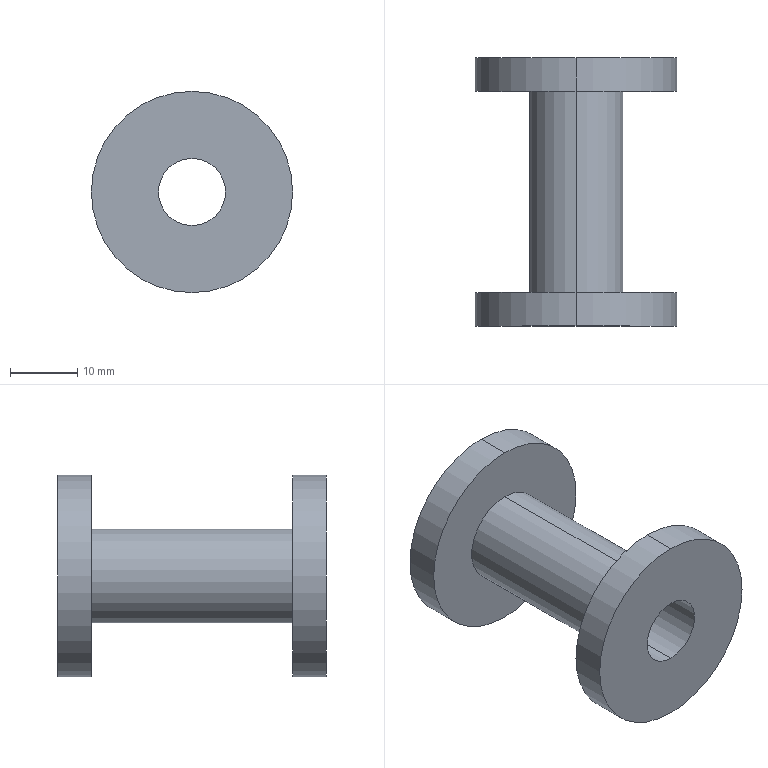Part | STEP file | inner coil1 | 1 solid | 12 faces | box 30 x 40 x 30 mm | volume 8545 mm3 | cylinder 8 | plane 4 | commonest cylinder face diameters 30 x4 10 x2 14 x2
STEP:
#1=CARTESIAN_POINT('',(0.,-15.,7.));
#2=VERTEX_POINT('',#1);
#3=CARTESIAN_POINT('',(0.,-15.,-7.));
#4=VERTEX_POINT('',#3);
#5=CARTESIAN_POINT('',(0.,-15.,0.));
#6=DIRECTION('',(0.,1.,0.));
#7=DIRECTION('',(0.,0.,1.));
#8=AXIS2_PLACEMENT_3D('',#5,#6,#7);
#9=CIRCLE('',#8,7.);
#10=EDGE_CURVE('',#2,#4,#9,.T.);
#11=ORIENTED_EDGE('',*,*,#10,.T.);
#12=CARTESIAN_POINT('',(0.,15.,-7.));
#13=VERTEX_POINT('',#12);
#14=CARTESIAN_POINT('',(0.,13.555,-7.));
#15=DIRECTION('',(0.,1.,0.));
#16=VECTOR('',#15,1000.);
#17=LINE('',#14,#16);
#18=EDGE_CURVE('',#4,#13,#17,.T.);
#19=ORIENTED_EDGE('',*,*,#18,.T.);
#20=CARTESIAN_POINT('',(0.,15.,7.));
#21=VERTEX_POINT('',#20);
#22=CARTESIAN_POINT('',(0.,15.,0.));
#23=DIRECTION('',(0.,1.,0.));
#24=DIRECTION('',(0.,0.,1.));
#25=AXIS2_PLACEMENT_3D('',#22,#23,#24);
#26=CIRCLE('',#25,7.);
#27=EDGE_CURVE('',#21,#13,#26,.T.);
#28=ORIENTED_EDGE('',*,*,#27,.F.);
#29=CARTESIAN_POINT('',(0.,13.555,7.));
#30=DIRECTION('',(0.,1.,0.));
#31=VECTOR('',#30,1000.);
#32=LINE('',#29,#31);
#33=EDGE_CURVE('',#2,#21,#32,.T.);
#34=ORIENTED_EDGE('',*,*,#33,.F.);
#35=EDGE_LOOP('',(#11,#19,#28,#34));
#36=FACE_OUTER_BOUND('',#35,.T.);
#37=CARTESIAN_POINT('',(0.,13.555,0.));
#38=DIRECTION('',(0.,1.,0.));
#39=DIRECTION('',(0.,0.,1.));
#40=AXIS2_PLACEMENT_3D('',#37,#38,#39);
#41=CYLINDRICAL_SURFACE('',#40,7.);
#42=ADVANCED_FACE('',(#36),#41,.T.);
#43=CARTESIAN_POINT('',(0.,-20.,-5.));
#44=VERTEX_POINT('',#43);
#45=CARTESIAN_POINT('',(0.,-20.,5.));
#46=VERTEX_POINT('',#45);
#47=CARTESIAN_POINT('',(0.,-20.,0.));
#48=DIRECTION('',(0.,1.,0.));
#49=DIRECTION('',(0.,0.,1.));
#50=AXIS2_PLACEMENT_3D('',#47,#48,#49);
#51=CIRCLE('',#50,5.);
#52=EDGE_CURVE('',#44,#46,#51,.T.);
#53=ORIENTED_EDGE('',*,*,#52,.F.);
#54=CARTESIAN_POINT('',(0.,20.,-5.));
#55=VERTEX_POINT('',#54);
#56=CARTESIAN_POINT('',(0.,65.771,-5.));
#57=DIRECTION('',(0.,1.,0.));
#58=VECTOR('',#57,1000.);
#59=LINE('',#56,#58);
#60=EDGE_CURVE('',#44,#55,#59,.T.);
#61=ORIENTED_EDGE('',*,*,#60,.T.);
#62=CARTESIAN_POINT('',(0.,20.,5.));
#63=VERTEX_POINT('',#62);
#64=CARTESIAN_POINT('',(0.,20.,0.));
#65=DIRECTION('',(0.,1.,0.));
#66=DIRECTION('',(0.,0.,1.));
#67=AXIS2_PLACEMENT_3D('',#64,#65,#66);
#68=CIRCLE('',#67,5.);
#69=EDGE_CURVE('',#55,#63,#68,.T.);
#70=ORIENTED_EDGE('',*,*,#69,.T.);
#71=CARTESIAN_POINT('',(0.,65.771,5.));
#72=DIRECTION('',(0.,1.,0.));
#73=VECTOR('',#72,1000.);
#74=LINE('',#71,#73);
#75=EDGE_CURVE('',#46,#63,#74,.T.);
#76=ORIENTED_EDGE('',*,*,#75,.F.);
#77=EDGE_LOOP('',(#53,#61,#70,#76));
#78=FACE_OUTER_BOUND('',#77,.T.);
#79=CARTESIAN_POINT('',(0.,65.771,0.));
#80=DIRECTION('',(0.,1.,0.));
#81=DIRECTION('',(0.,0.,1.));
#82=AXIS2_PLACEMENT_3D('',#79,#80,#81);
#83=CYLINDRICAL_SURFACE('',#82,5.);
#84=ADVANCED_FACE('',(#78),#83,.F.);
#85=CARTESIAN_POINT('',(0.,15.,15.));
#86=VERTEX_POINT('',#85);
#87=CARTESIAN_POINT('',(0.,15.,-15.));
#88=VERTEX_POINT('',#87);
#89=CARTESIAN_POINT('',(0.,15.,0.));
#90=DIRECTION('',(0.,1.,0.));
#91=DIRECTION('',(0.,0.,1.));
#92=AXIS2_PLACEMENT_3D('',#89,#90,#91);
#93=CIRCLE('',#92,15.);
#94=EDGE_CURVE('',#86,#88,#93,.T.);
#95=ORIENTED_EDGE('',*,*,#94,.T.);
#96=CARTESIAN_POINT('',(0.,20.,-15.));
#97=VERTEX_POINT('',#96);
#98=CARTESIAN_POINT('',(0.,65.771,-15.));
#99=DIRECTION('',(0.,1.,0.));
#100=VECTOR('',#99,1000.);
#101=LINE('',#98,#100);
#102=EDGE_CURVE('',#88,#97,#101,.T.);
#103=ORIENTED_EDGE('',*,*,#102,.T.);
#104=CARTESIAN_POINT('',(0.,20.,15.));
#105=VERTEX_POINT('',#104);
#106=CARTESIAN_POINT('',(0.,20.,0.));
#107=DIRECTION('',(0.,1.,0.));
#108=DIRECTION('',(0.,0.,1.));
#109=AXIS2_PLACEMENT_3D('',#106,#107,#108);
#110=CIRCLE('',#109,15.);
#111=EDGE_CURVE('',#105,#97,#110,.T.);
#112=ORIENTED_EDGE('',*,*,#111,.F.);
#113=CARTESIAN_POINT('',(0.,65.771,15.));
#114=DIRECTION('',(0.,1.,0.));
#115=VECTOR('',#114,1000.);
#116=LINE('',#113,#115);
#117=EDGE_CURVE('',#86,#105,#116,.T.);
#118=ORIENTED_EDGE('',*,*,#117,.F.);
#119=EDGE_LOOP('',(#95,#103,#112,#118));
#120=FACE_OUTER_BOUND('',#119,.T.);
#121=CARTESIAN_POINT('',(0.,65.771,0.));
#122=DIRECTION('',(0.,1.,0.));
#123=DIRECTION('',(0.,0.,1.));
#124=AXIS2_PLACEMENT_3D('',#121,#122,#123);
#125=CYLINDRICAL_SURFACE('',#124,15.);
#126=ADVANCED_FACE('',(#120),#125,.T.);
#127=CARTESIAN_POINT('',(0.,-20.,15.));
#128=VERTEX_POINT('',#127);
#129=CARTESIAN_POINT('',(0.,-20.,-15.));
#130=VERTEX_POINT('',#129);
#131=CARTESIAN_POINT('',(0.,-20.,0.));
#132=DIRECTION('',(0.,1.,0.));
#133=DIRECTION('',(0.,0.,1.));
#134=AXIS2_PLACEMENT_3D('',#131,#132,#133);
#135=CIRCLE('',#134,15.);
#136=EDGE_CURVE('',#128,#130,#135,.T.);
#137=ORIENTED_EDGE('',*,*,#136,.T.);
#138=CARTESIAN_POINT('',(0.,-15.,-15.));
#139=VERTEX_POINT('',#138);
#140=CARTESIAN_POINT('',(0.,65.771,-15.));
#141=DIRECTION('',(0.,1.,0.));
#142=VECTOR('',#141,1000.);
#143=LINE('',#140,#142);
#144=EDGE_CURVE('',#130,#139,#143,.T.);
#145=ORIENTED_EDGE('',*,*,#144,.T.);
#146=CARTESIAN_POINT('',(0.,-15.,15.));
#147=VERTEX_POINT('',#146);
#148=CARTESIAN_POINT('',(0.,-15.,0.));
#149=DIRECTION('',(0.,1.,0.));
#150=DIRECTION('',(0.,0.,1.));
#151=AXIS2_PLACEMENT_3D('',#148,#149,#150);
#152=CIRCLE('',#151,15.);
#153=EDGE_CURVE('',#147,#139,#152,.T.);
#154=ORIENTED_EDGE('',*,*,#153,.F.);
#155=CARTESIAN_POINT('',(0.,65.771,15.));
#156=DIRECTION('',(0.,1.,0.));
#157=VECTOR('',#156,1000.);
#158=LINE('',#155,#157);
#159=EDGE_CURVE('',#128,#147,#158,.T.);
#160=ORIENTED_EDGE('',*,*,#159,.F.);
#161=EDGE_LOOP('',(#137,#145,#154,#160));
#162=FACE_OUTER_BOUND('',#161,.T.);
#163=CARTESIAN_POINT('',(0.,65.771,0.));
#164=DIRECTION('',(0.,1.,0.));
#165=DIRECTION('',(0.,0.,1.));
#166=AXIS2_PLACEMENT_3D('',#163,#164,#165);
#167=CYLINDRICAL_SURFACE('',#166,15.);
#168=ADVANCED_FACE('',(#162),#167,.T.);
#169=ORIENTED_EDGE('',*,*,#144,.F.);
#170=CARTESIAN_POINT('',(0.,-20.,0.));
#171=DIRECTION('',(0.,1.,0.));
#172=DIRECTION('',(0.,0.,1.));
#173=AXIS2_PLACEMENT_3D('',#170,#171,#172);
#174=CIRCLE('',#173,15.);
#175=EDGE_CURVE('',#130,#128,#174,.T.);
#176=ORIENTED_EDGE('',*,*,#175,.T.);
#177=ORIENTED_EDGE('',*,*,#159,.T.);
#178=CARTESIAN_POINT('',(0.,-15.,0.));
#179=DIRECTION('',(0.,1.,0.));
#180=DIRECTION('',(0.,0.,1.));
#181=AXIS2_PLACEMENT_3D('',#178,#179,#180);
#182=CIRCLE('',#181,15.);
#183=EDGE_CURVE('',#139,#147,#182,.T.);
#184=ORIENTED_EDGE('',*,*,#183,.F.);
#185=EDGE_LOOP('',(#169,#176,#177,#184));
#186=FACE_OUTER_BOUND('',#185,.T.);
#187=CARTESIAN_POINT('',(0.,65.771,0.));
#188=DIRECTION('',(0.,1.,0.));
#189=DIRECTION('',(0.,0.,1.));
#190=AXIS2_PLACEMENT_3D('',#187,#188,#189);
#191=CYLINDRICAL_SURFACE('',#190,15.);
#192=ADVANCED_FACE('',(#186),#191,.T.);
#193=ORIENTED_EDGE('',*,*,#102,.F.);
#194=CARTESIAN_POINT('',(0.,15.,0.));
#195=DIRECTION('',(0.,1.,0.));
#196=DIRECTION('',(0.,0.,1.));
#197=AXIS2_PLACEMENT_3D('',#194,#195,#196);
#198=CIRCLE('',#197,15.);
#199=EDGE_CURVE('',#88,#86,#198,.T.);
#200=ORIENTED_EDGE('',*,*,#199,.T.);
#201=ORIENTED_EDGE('',*,*,#117,.T.);
#202=CARTESIAN_POINT('',(0.,20.,0.));
#203=DIRECTION('',(0.,1.,0.));
#204=DIRECTION('',(0.,0.,1.));
#205=AXIS2_PLACEMENT_3D('',#202,#203,#204);
#206=CIRCLE('',#205,15.);
#207=EDGE_CURVE('',#97,#105,#206,.T.);
#208=ORIENTED_EDGE('',*,*,#207,.F.);
#209=EDGE_LOOP('',(#193,#200,#201,#208));
#210=FACE_OUTER_BOUND('',#209,.T.);
#211=CARTESIAN_POINT('',(0.,65.771,0.));
#212=DIRECTION('',(0.,1.,0.));
#213=DIRECTION('',(0.,0.,1.));
#214=AXIS2_PLACEMENT_3D('',#211,#212,#213);
#215=CYLINDRICAL_SURFACE('',#214,15.);
#216=ADVANCED_FACE('',(#210),#215,.T.);
#217=ORIENTED_EDGE('',*,*,#111,.T.);
#218=ORIENTED_EDGE('',*,*,#207,.T.);
#219=EDGE_LOOP('',(#217,#218));
#220=FACE_OUTER_BOUND('',#219,.T.);
#221=CARTESIAN_POINT('',(0.,20.,0.));
#222=DIRECTION('',(0.,1.,0.));
#223=DIRECTION('',(0.,0.,1.));
#224=AXIS2_PLACEMENT_3D('',#221,#222,#223);
#225=CIRCLE('',#224,5.);
#226=EDGE_CURVE('',#63,#55,#225,.T.);
#227=ORIENTED_EDGE('',*,*,#226,.F.);
#228=ORIENTED_EDGE('',*,*,#69,.F.);
#229=EDGE_LOOP('',(#227,#228));
#230=FACE_BOUND('',#229,.T.);
#231=CARTESIAN_POINT('',(-5.,20.,0.));
#232=DIRECTION('',(0.,1.,0.));
#233=DIRECTION('',(0.,0.,1.));
#234=AXIS2_PLACEMENT_3D('',#231,#232,#233);
#235=PLANE('',#234);
#236=ADVANCED_FACE('',(#220,#230),#235,.T.);
#237=ORIENTED_EDGE('',*,*,#60,.F.);
#238=CARTESIAN_POINT('',(0.,-20.,0.));
#239=DIRECTION('',(0.,1.,0.));
#240=DIRECTION('',(0.,0.,1.));
#241=AXIS2_PLACEMENT_3D('',#238,#239,#240);
#242=CIRCLE('',#241,5.);
#243=EDGE_CURVE('',#46,#44,#242,.T.);
#244=ORIENTED_EDGE('',*,*,#243,.F.);
#245=ORIENTED_EDGE('',*,*,#75,.T.);
#246=ORIENTED_EDGE('',*,*,#226,.T.);
#247=EDGE_LOOP('',(#237,#244,#245,#246));
#248=FACE_OUTER_BOUND('',#247,.T.);
#249=CARTESIAN_POINT('',(0.,65.771,0.));
#250=DIRECTION('',(0.,1.,0.));
#251=DIRECTION('',(0.,0.,1.));
#252=AXIS2_PLACEMENT_3D('',#249,#250,#251);
#253=CYLINDRICAL_SURFACE('',#252,5.);
#254=ADVANCED_FACE('',(#248),#253,.F.);
#255=ORIENTED_EDGE('',*,*,#243,.T.);
#256=ORIENTED_EDGE('',*,*,#52,.T.);
#257=EDGE_LOOP('',(#255,#256));
#258=FACE_BOUND('',#257,.T.);
#259=ORIENTED_EDGE('',*,*,#136,.F.);
#260=ORIENTED_EDGE('',*,*,#175,.F.);
#261=EDGE_LOOP('',(#259,#260));
#262=FACE_OUTER_BOUND('',#261,.T.);
#263=CARTESIAN_POINT('',(-5.,-20.,0.));
#264=DIRECTION('',(0.,-1.,0.));
#265=DIRECTION('',(0.,0.,-1.));
#266=AXIS2_PLACEMENT_3D('',#263,#264,#265);
#267=PLANE('',#266);
#268=ADVANCED_FACE('',(#258,#262),#267,.T.);
#269=ORIENTED_EDGE('',*,*,#10,.F.);
#270=CARTESIAN_POINT('',(0.,-15.,0.));
#271=DIRECTION('',(0.,1.,0.));
#272=DIRECTION('',(0.,0.,1.));
#273=AXIS2_PLACEMENT_3D('',#270,#271,#272);
#274=CIRCLE('',#273,7.);
#275=EDGE_CURVE('',#4,#2,#274,.T.);
#276=ORIENTED_EDGE('',*,*,#275,.F.);
#277=EDGE_LOOP('',(#269,#276));
#278=FACE_BOUND('',#277,.T.);
#279=ORIENTED_EDGE('',*,*,#153,.T.);
#280=ORIENTED_EDGE('',*,*,#183,.T.);
#281=EDGE_LOOP('',(#279,#280));
#282=FACE_OUTER_BOUND('',#281,.T.);
#283=CARTESIAN_POINT('',(-7.,-15.,0.));
#284=DIRECTION('',(0.,-1.,0.));
#285=DIRECTION('',(0.,0.,-1.));
#286=AXIS2_PLACEMENT_3D('',#283,#284,#285);
#287=PLANE('',#286);
#288=ADVANCED_FACE('',(#278,#282),#287,.F.);
#289=ORIENTED_EDGE('',*,*,#18,.F.);
#290=ORIENTED_EDGE('',*,*,#275,.T.);
#291=ORIENTED_EDGE('',*,*,#33,.T.);
#292=CARTESIAN_POINT('',(0.,15.,0.));
#293=DIRECTION('',(0.,1.,0.));
#294=DIRECTION('',(0.,0.,1.));
#295=AXIS2_PLACEMENT_3D('',#292,#293,#294);
#296=CIRCLE('',#295,7.);
#297=EDGE_CURVE('',#13,#21,#296,.T.);
#298=ORIENTED_EDGE('',*,*,#297,.F.);
#299=EDGE_LOOP('',(#289,#290,#291,#298));
#300=FACE_OUTER_BOUND('',#299,.T.);
#301=CARTESIAN_POINT('',(0.,13.555,0.));
#302=DIRECTION('',(0.,1.,0.));
#303=DIRECTION('',(0.,0.,1.));
#304=AXIS2_PLACEMENT_3D('',#301,#302,#303);
#305=CYLINDRICAL_SURFACE('',#304,7.);
#306=ADVANCED_FACE('',(#300),#305,.T.);
#307=ORIENTED_EDGE('',*,*,#94,.F.);
#308=ORIENTED_EDGE('',*,*,#199,.F.);
#309=EDGE_LOOP('',(#307,#308));
#310=FACE_OUTER_BOUND('',#309,.T.);
#311=ORIENTED_EDGE('',*,*,#27,.T.);
#312=ORIENTED_EDGE('',*,*,#297,.T.);
#313=EDGE_LOOP('',(#311,#312));
#314=FACE_BOUND('',#313,.T.);
#315=CARTESIAN_POINT('',(-7.,15.,0.));
#316=DIRECTION('',(0.,1.,0.));
#317=DIRECTION('',(0.,0.,1.));
#318=AXIS2_PLACEMENT_3D('',#315,#316,#317);
#319=PLANE('',#318);
#320=ADVANCED_FACE('',(#310,#314),#319,.F.);
#321=CLOSED_SHELL('',(#42,#84,#126,#168,#192,#216,#236,#254,#268,#288,#306,#320));
#322=MANIFOLD_SOLID_BREP('',#321);
#323=CARTESIAN_POINT('',(0.,0.,0.));
#324=DIRECTION('',(0.,0.,1.));
#325=DIRECTION('',(1.,0.,0.));
#326=AXIS2_PLACEMENT_3D('',#323,#324,#325);
#327=(LENGTH_UNIT()NAMED_UNIT(*)SI_UNIT(.MILLI.,.METRE.));
#328=UNCERTAINTY_MEASURE_WITH_UNIT(LENGTH_MEASURE(0.00001),#327,'','');
#329=(NAMED_UNIT(*)PLANE_ANGLE_UNIT()SI_UNIT($,.RADIAN.));
#330=(NAMED_UNIT(*)SI_UNIT($,.STERADIAN.)SOLID_ANGLE_UNIT());
#331=(GEOMETRIC_REPRESENTATION_CONTEXT(3)GLOBAL_UNCERTAINTY_ASSIGNED_CONTEXT((#328))GLOBAL_UNIT_ASSIGNED_CONTEXT((#327,#329,#330))REPRESENTATION_CONTEXT('',''));
#332=ADVANCED_BREP_SHAPE_REPRESENTATION('',(#322,#326),#331);